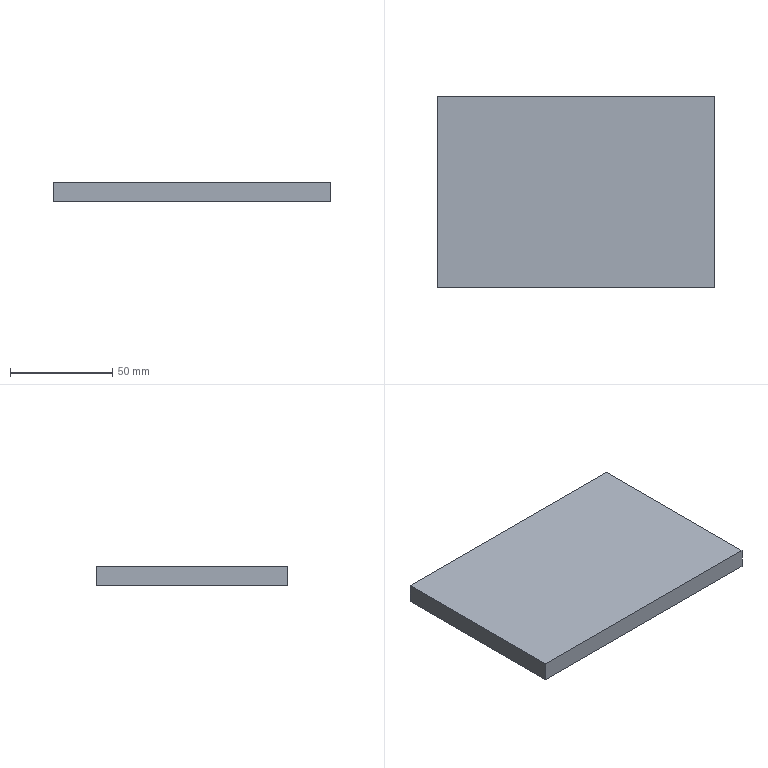Part | NX | features 打孔尺寸(%根据)内六角圆柱头螺钉的类型1 2 | 1 solid | 6 faces | box 136 x 94 x 9.5 mm | volume 121448 mm3 | plane 6
STEP:
#1=CARTESIAN_POINT('',(-68.,129.,-121.));
#2=VERTEX_POINT('',#1);
#3=CARTESIAN_POINT('',(-68.,35.,-121.));
#4=VERTEX_POINT('',#3);
#5=CARTESIAN_POINT('',(-68.,122.,-121.));
#6=DIRECTION('',(0.,-1.,0.));
#7=VECTOR('',#6,1000.);
#8=LINE('',#5,#7);
#9=EDGE_CURVE('',#2,#4,#8,.T.);
#10=ORIENTED_EDGE('',*,*,#9,.T.);
#11=CARTESIAN_POINT('',(-68.,35.,-111.5));
#12=VERTEX_POINT('',#11);
#13=CARTESIAN_POINT('',(-68.,35.,-101.5));
#14=DIRECTION('',(0.,0.,-1.));
#15=VECTOR('',#14,1000.);
#16=LINE('',#13,#15);
#17=EDGE_CURVE('',#12,#4,#16,.T.);
#18=ORIENTED_EDGE('',*,*,#17,.F.);
#19=CARTESIAN_POINT('',(-68.,129.,-111.5));
#20=VERTEX_POINT('',#19);
#21=CARTESIAN_POINT('',(-68.,122.,-111.5));
#22=DIRECTION('',(0.,1.,0.));
#23=VECTOR('',#22,1000.);
#24=LINE('',#21,#23);
#25=EDGE_CURVE('',#20,#12,#24,.F.);
#26=ORIENTED_EDGE('',*,*,#25,.F.);
#27=CARTESIAN_POINT('',(-68.,129.,-82.5));
#28=DIRECTION('',(0.,0.,1.));
#29=VECTOR('',#28,1000.);
#30=LINE('',#27,#29);
#31=EDGE_CURVE('',#20,#2,#30,.F.);
#32=ORIENTED_EDGE('',*,*,#31,.T.);
#33=EDGE_LOOP('',(#10,#18,#26,#32));
#34=FACE_BOUND('',#33,.T.);
#35=CARTESIAN_POINT('',(-68.,122.,-82.5));
#36=DIRECTION('',(1.,0.,0.));
#37=DIRECTION('',(0.,0.,-1.));
#38=AXIS2_PLACEMENT_3D('',#35,#36,#37);
#39=PLANE('',#38);
#40=ADVANCED_FACE('',(#34),#39,.F.);
#41=CARTESIAN_POINT('',(68.,35.,-121.));
#42=VERTEX_POINT('',#41);
#43=CARTESIAN_POINT('',(35.,35.,-121.));
#44=DIRECTION('',(1.,0.,0.));
#45=VECTOR('',#44,1000.);
#46=LINE('',#43,#45);
#47=EDGE_CURVE('',#4,#42,#46,.T.);
#48=ORIENTED_EDGE('',*,*,#47,.T.);
#49=CARTESIAN_POINT('',(68.,35.,-111.5));
#50=VERTEX_POINT('',#49);
#51=CARTESIAN_POINT('',(68.,35.,-82.5));
#52=DIRECTION('',(0.,0.,-1.));
#53=VECTOR('',#52,1000.);
#54=LINE('',#51,#53);
#55=EDGE_CURVE('',#50,#42,#54,.T.);
#56=ORIENTED_EDGE('',*,*,#55,.F.);
#57=CARTESIAN_POINT('',(35.,35.,-111.5));
#58=DIRECTION('',(-1.,0.,-0.000000009));
#59=VECTOR('',#58,1000.);
#60=LINE('',#57,#59);
#61=EDGE_CURVE('',#12,#50,#60,.F.);
#62=ORIENTED_EDGE('',*,*,#61,.F.);
#63=ORIENTED_EDGE('',*,*,#17,.T.);
#64=EDGE_LOOP('',(#48,#56,#62,#63));
#65=FACE_BOUND('',#64,.T.);
#66=CARTESIAN_POINT('',(35.,35.,-101.5));
#67=DIRECTION('',(0.,1.,0.));
#68=DIRECTION('',(0.977,0.,0.2131));
#69=AXIS2_PLACEMENT_3D('',#66,#67,#68);
#70=PLANE('',#69);
#71=ADVANCED_FACE('',(#65),#70,.F.);
#72=CARTESIAN_POINT('',(68.,129.,-121.));
#73=VERTEX_POINT('',#72);
#74=CARTESIAN_POINT('',(68.,76.,-121.));
#75=DIRECTION('',(0.,1.,0.));
#76=VECTOR('',#75,1000.);
#77=LINE('',#74,#76);
#78=EDGE_CURVE('',#42,#73,#77,.T.);
#79=ORIENTED_EDGE('',*,*,#78,.T.);
#80=CARTESIAN_POINT('',(68.,129.,-111.5));
#81=VERTEX_POINT('',#80);
#82=CARTESIAN_POINT('',(68.,129.,-122.5));
#83=DIRECTION('',(0.,0.,1.));
#84=VECTOR('',#83,1000.);
#85=LINE('',#82,#84);
#86=EDGE_CURVE('',#81,#73,#85,.F.);
#87=ORIENTED_EDGE('',*,*,#86,.F.);
#88=CARTESIAN_POINT('',(68.,76.,-111.5));
#89=DIRECTION('',(0.,-1.,0.));
#90=VECTOR('',#89,1000.);
#91=LINE('',#88,#90);
#92=EDGE_CURVE('',#50,#81,#91,.F.);
#93=ORIENTED_EDGE('',*,*,#92,.F.);
#94=ORIENTED_EDGE('',*,*,#55,.T.);
#95=EDGE_LOOP('',(#79,#87,#93,#94));
#96=FACE_BOUND('',#95,.T.);
#97=CARTESIAN_POINT('',(68.,76.,-82.5));
#98=DIRECTION('',(-1.,0.,0.));
#99=DIRECTION('',(0.,0.,-1.));
#100=AXIS2_PLACEMENT_3D('',#97,#98,#99);
#101=PLANE('',#100);
#102=ADVANCED_FACE('',(#96),#101,.F.);
#103=CARTESIAN_POINT('',(50.,129.,-121.));
#104=DIRECTION('',(1.,0.,0.));
#105=VECTOR('',#104,1000.);
#106=LINE('',#103,#105);
#107=EDGE_CURVE('',#73,#2,#106,.F.);
#108=ORIENTED_EDGE('',*,*,#107,.T.);
#109=ORIENTED_EDGE('',*,*,#31,.F.);
#110=CARTESIAN_POINT('',(50.,129.,-111.5));
#111=DIRECTION('',(-1.,0.,-0.000000009));
#112=VECTOR('',#111,1000.);
#113=LINE('',#110,#112);
#114=EDGE_CURVE('',#81,#20,#113,.T.);
#115=ORIENTED_EDGE('',*,*,#114,.F.);
#116=ORIENTED_EDGE('',*,*,#86,.T.);
#117=EDGE_LOOP('',(#108,#109,#115,#116));
#118=FACE_BOUND('',#117,.T.);
#119=CARTESIAN_POINT('',(50.,129.,-122.5));
#120=DIRECTION('',(0.,1.,0.));
#121=DIRECTION('',(0.,0.,1.));
#122=AXIS2_PLACEMENT_3D('',#119,#120,#121);
#123=PLANE('',#122);
#124=ADVANCED_FACE('',(#118),#123,.T.);
#125=ORIENTED_EDGE('',*,*,#25,.T.);
#126=ORIENTED_EDGE('',*,*,#61,.T.);
#127=ORIENTED_EDGE('',*,*,#92,.T.);
#128=ORIENTED_EDGE('',*,*,#114,.T.);
#129=EDGE_LOOP('',(#125,#126,#127,#128));
#130=FACE_BOUND('',#129,.T.);
#131=CARTESIAN_POINT('',(15.,99.3,-111.5));
#132=DIRECTION('',(0.000000009,0.,-1.));
#133=DIRECTION('',(0.,1.,0.));
#134=AXIS2_PLACEMENT_3D('',#131,#132,#133);
#135=PLANE('',#134);
#136=ADVANCED_FACE('',(#130),#135,.F.);
#137=ORIENTED_EDGE('',*,*,#9,.F.);
#138=ORIENTED_EDGE('',*,*,#107,.F.);
#139=ORIENTED_EDGE('',*,*,#78,.F.);
#140=ORIENTED_EDGE('',*,*,#47,.F.);
#141=EDGE_LOOP('',(#137,#138,#139,#140));
#142=FACE_BOUND('',#141,.T.);
#143=CARTESIAN_POINT('',(1.,-14.,-121.));
#144=DIRECTION('',(0.,0.,1.));
#145=DIRECTION('',(1.,0.,0.));
#146=AXIS2_PLACEMENT_3D('',#143,#144,#145);
#147=PLANE('',#146);
#148=ADVANCED_FACE('',(#142),#147,.F.);
#149=CLOSED_SHELL('',(#40,#71,#102,#124,#136,#148));
#150=MANIFOLD_SOLID_BREP('',#149);
#151=(LENGTH_UNIT()NAMED_UNIT(*)SI_UNIT(.MILLI.,.METRE.));
#152=UNCERTAINTY_MEASURE_WITH_UNIT(LENGTH_MEASURE(0.00001),#151,'','');
#153=(NAMED_UNIT(*)PLANE_ANGLE_UNIT()SI_UNIT($,.RADIAN.));
#154=(NAMED_UNIT(*)SI_UNIT($,.STERADIAN.)SOLID_ANGLE_UNIT());
#155=(GEOMETRIC_REPRESENTATION_CONTEXT(3)GLOBAL_UNCERTAINTY_ASSIGNED_CONTEXT((#152))GLOBAL_UNIT_ASSIGNED_CONTEXT((#151,#153,#154))REPRESENTATION_CONTEXT('',''));
#156=ADVANCED_BREP_SHAPE_REPRESENTATION('',(#150),#155);